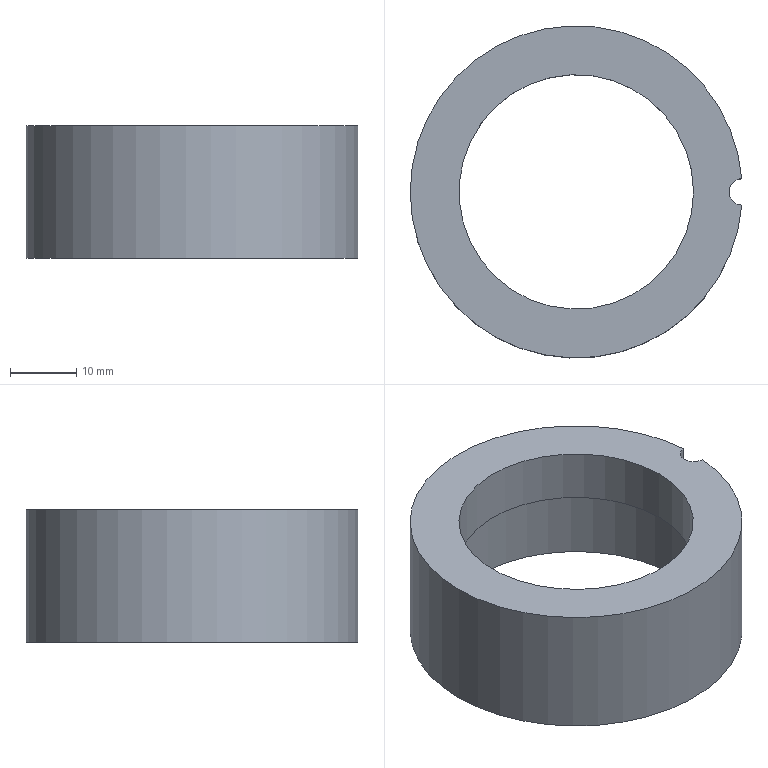Part | NX | features solid 2 | 1 solid | 7 faces | box 49.92 x 50 x 20 mm | volume 15474 mm3 | cylinder 4 | plane 3 | commonest cylinder face diameters 4 x1 35.3 x1 41 x1 50 x1
STEP:
#1=CARTESIAN_POINT('',(-812.565,-167.669,54.));
#2=VERTEX_POINT('',#1);
#3=CARTESIAN_POINT('',(-812.565,-167.669,74.));
#4=VERTEX_POINT('',#3);
#5=CARTESIAN_POINT('',(-812.565,-167.669,64.));
#6=DIRECTION('',(0.,0.,1.));
#7=VECTOR('',#6,1000.);
#8=LINE('',#5,#7);
#9=EDGE_CURVE('',#2,#4,#8,.T.);
#10=ORIENTED_EDGE('',*,*,#9,.F.);
#11=CARTESIAN_POINT('',(-812.565,-171.666,54.));
#12=VERTEX_POINT('',#11);
#13=CARTESIAN_POINT('',(-837.485,-169.668,54.));
#14=DIRECTION('',(0.,0.,1.));
#15=DIRECTION('',(1.,0.,0.));
#16=AXIS2_PLACEMENT_3D('',#13,#14,#15);
#17=CIRCLE('',#16,25.);
#18=EDGE_CURVE('',#2,#12,#17,.T.);
#19=ORIENTED_EDGE('',*,*,#18,.T.);
#20=CARTESIAN_POINT('',(-812.565,-171.666,74.));
#21=VERTEX_POINT('',#20);
#22=CARTESIAN_POINT('',(-812.565,-171.666,64.));
#23=DIRECTION('',(0.,0.,1.));
#24=VECTOR('',#23,1000.);
#25=LINE('',#22,#24);
#26=EDGE_CURVE('',#21,#12,#25,.F.);
#27=ORIENTED_EDGE('',*,*,#26,.F.);
#28=CARTESIAN_POINT('',(-837.485,-169.668,74.));
#29=DIRECTION('',(0.,0.,1.));
#30=DIRECTION('',(1.,0.,0.));
#31=AXIS2_PLACEMENT_3D('',#28,#29,#30);
#32=CIRCLE('',#31,25.);
#33=EDGE_CURVE('',#4,#21,#32,.T.);
#34=ORIENTED_EDGE('',*,*,#33,.F.);
#35=EDGE_LOOP('',(#10,#19,#27,#34));
#36=FACE_BOUND('',#35,.T.);
#37=CARTESIAN_POINT('',(-837.485,-169.668,54.));
#38=DIRECTION('',(0.,0.,1.));
#39=DIRECTION('',(1.,0.,0.));
#40=AXIS2_PLACEMENT_3D('',#37,#38,#39);
#41=CYLINDRICAL_SURFACE('',#40,25.);
#42=ADVANCED_FACE('',(#36),#41,.T.);
#43=CARTESIAN_POINT('',(-816.985,-169.668,54.));
#44=VERTEX_POINT('',#43);
#45=CARTESIAN_POINT('',(-837.485,-169.668,54.));
#46=DIRECTION('',(0.,0.,1.));
#47=DIRECTION('',(1.,0.,0.));
#48=AXIS2_PLACEMENT_3D('',#45,#46,#47);
#49=CIRCLE('',#48,20.5);
#50=EDGE_CURVE('',#44,#44,#49,.T.);
#51=ORIENTED_EDGE('',*,*,#50,.T.);
#52=EDGE_LOOP('',(#51));
#53=FACE_BOUND('',#52,.T.);
#54=ORIENTED_EDGE('',*,*,#18,.F.);
#55=CARTESIAN_POINT('',(-812.485,-169.668,54.));
#56=DIRECTION('',(0.,0.,1.));
#57=DIRECTION('',(1.,0.,0.));
#58=AXIS2_PLACEMENT_3D('',#55,#56,#57);
#59=CIRCLE('',#58,2.);
#60=EDGE_CURVE('',#2,#12,#59,.T.);
#61=ORIENTED_EDGE('',*,*,#60,.T.);
#62=EDGE_LOOP('',(#54,#61));
#63=FACE_BOUND('',#62,.T.);
#64=CARTESIAN_POINT('',(-837.485,-169.668,54.));
#65=DIRECTION('',(0.,0.,1.));
#66=DIRECTION('',(1.,0.,0.));
#67=AXIS2_PLACEMENT_3D('',#64,#65,#66);
#68=PLANE('',#67);
#69=ADVANCED_FACE('',(#53,#63),#68,.F.);
#70=CARTESIAN_POINT('',(-819.835,-169.668,74.));
#71=VERTEX_POINT('',#70);
#72=CARTESIAN_POINT('',(-837.485,-169.668,74.));
#73=DIRECTION('',(0.,0.,1.));
#74=DIRECTION('',(1.,0.,0.));
#75=AXIS2_PLACEMENT_3D('',#72,#73,#74);
#76=CIRCLE('',#75,17.65);
#77=EDGE_CURVE('',#71,#71,#76,.T.);
#78=ORIENTED_EDGE('',*,*,#77,.F.);
#79=EDGE_LOOP('',(#78));
#80=FACE_BOUND('',#79,.T.);
#81=CARTESIAN_POINT('',(-812.485,-169.668,74.));
#82=DIRECTION('',(0.,0.,1.));
#83=DIRECTION('',(1.,0.,0.));
#84=AXIS2_PLACEMENT_3D('',#81,#82,#83);
#85=CIRCLE('',#84,2.);
#86=EDGE_CURVE('',#4,#21,#85,.T.);
#87=ORIENTED_EDGE('',*,*,#86,.F.);
#88=ORIENTED_EDGE('',*,*,#33,.T.);
#89=EDGE_LOOP('',(#87,#88));
#90=FACE_BOUND('',#89,.T.);
#91=CARTESIAN_POINT('',(-837.485,-169.668,74.));
#92=DIRECTION('',(0.,0.,1.));
#93=DIRECTION('',(1.,0.,0.));
#94=AXIS2_PLACEMENT_3D('',#91,#92,#93);
#95=PLANE('',#94);
#96=ADVANCED_FACE('',(#80,#90),#95,.T.);
#97=ORIENTED_EDGE('',*,*,#50,.F.);
#98=EDGE_LOOP('',(#97));
#99=FACE_BOUND('',#98,.T.);
#100=CARTESIAN_POINT('',(-816.985,-169.668,66.));
#101=VERTEX_POINT('',#100);
#102=CARTESIAN_POINT('',(-837.485,-169.668,66.));
#103=DIRECTION('',(0.,0.,1.));
#104=DIRECTION('',(1.,0.,0.));
#105=AXIS2_PLACEMENT_3D('',#102,#103,#104);
#106=CIRCLE('',#105,20.5);
#107=EDGE_CURVE('',#101,#101,#106,.T.);
#108=ORIENTED_EDGE('',*,*,#107,.T.);
#109=EDGE_LOOP('',(#108));
#110=FACE_BOUND('',#109,.T.);
#111=CARTESIAN_POINT('',(-837.485,-169.668,54.));
#112=DIRECTION('',(0.,0.,1.));
#113=DIRECTION('',(1.,0.,0.));
#114=AXIS2_PLACEMENT_3D('',#111,#112,#113);
#115=CYLINDRICAL_SURFACE('',#114,20.5);
#116=ADVANCED_FACE('',(#99,#110),#115,.F.);
#117=CARTESIAN_POINT('',(-819.835,-169.668,66.));
#118=VERTEX_POINT('',#117);
#119=CARTESIAN_POINT('',(-837.485,-169.668,66.));
#120=DIRECTION('',(0.,0.,1.));
#121=DIRECTION('',(1.,0.,0.));
#122=AXIS2_PLACEMENT_3D('',#119,#120,#121);
#123=CIRCLE('',#122,17.65);
#124=EDGE_CURVE('',#118,#118,#123,.T.);
#125=ORIENTED_EDGE('',*,*,#124,.T.);
#126=EDGE_LOOP('',(#125));
#127=FACE_BOUND('',#126,.T.);
#128=ORIENTED_EDGE('',*,*,#107,.F.);
#129=EDGE_LOOP('',(#128));
#130=FACE_BOUND('',#129,.T.);
#131=CARTESIAN_POINT('',(-837.485,-169.668,66.));
#132=DIRECTION('',(0.,0.,1.));
#133=DIRECTION('',(1.,0.,0.));
#134=AXIS2_PLACEMENT_3D('',#131,#132,#133);
#135=PLANE('',#134);
#136=ADVANCED_FACE('',(#127,#130),#135,.F.);
#137=ORIENTED_EDGE('',*,*,#9,.T.);
#138=ORIENTED_EDGE('',*,*,#86,.T.);
#139=ORIENTED_EDGE('',*,*,#26,.T.);
#140=ORIENTED_EDGE('',*,*,#60,.F.);
#141=EDGE_LOOP('',(#137,#138,#139,#140));
#142=FACE_BOUND('',#141,.T.);
#143=CARTESIAN_POINT('',(-812.485,-169.668,54.));
#144=DIRECTION('',(0.,0.,1.));
#145=DIRECTION('',(1.,0.,0.));
#146=AXIS2_PLACEMENT_3D('',#143,#144,#145);
#147=CYLINDRICAL_SURFACE('',#146,2.);
#148=ADVANCED_FACE('',(#142),#147,.F.);
#149=ORIENTED_EDGE('',*,*,#77,.T.);
#150=EDGE_LOOP('',(#149));
#151=FACE_BOUND('',#150,.T.);
#152=ORIENTED_EDGE('',*,*,#124,.F.);
#153=EDGE_LOOP('',(#152));
#154=FACE_BOUND('',#153,.T.);
#155=CARTESIAN_POINT('',(-837.485,-169.668,54.));
#156=DIRECTION('',(0.,0.,1.));
#157=DIRECTION('',(1.,0.,0.));
#158=AXIS2_PLACEMENT_3D('',#155,#156,#157);
#159=CYLINDRICAL_SURFACE('',#158,17.65);
#160=ADVANCED_FACE('',(#151,#154),#159,.F.);
#161=CLOSED_SHELL('',(#42,#69,#96,#116,#136,#148,#160));
#162=MANIFOLD_SOLID_BREP('',#161);
#163=(LENGTH_UNIT()NAMED_UNIT(*)SI_UNIT(.MILLI.,.METRE.));
#164=UNCERTAINTY_MEASURE_WITH_UNIT(LENGTH_MEASURE(0.00001),#163,'','');
#165=(NAMED_UNIT(*)PLANE_ANGLE_UNIT()SI_UNIT($,.RADIAN.));
#166=(NAMED_UNIT(*)SI_UNIT($,.STERADIAN.)SOLID_ANGLE_UNIT());
#167=(GEOMETRIC_REPRESENTATION_CONTEXT(3)GLOBAL_UNCERTAINTY_ASSIGNED_CONTEXT((#164))GLOBAL_UNIT_ASSIGNED_CONTEXT((#163,#165,#166))REPRESENTATION_CONTEXT('',''));
#168=ADVANCED_BREP_SHAPE_REPRESENTATION('',(#162),#167);